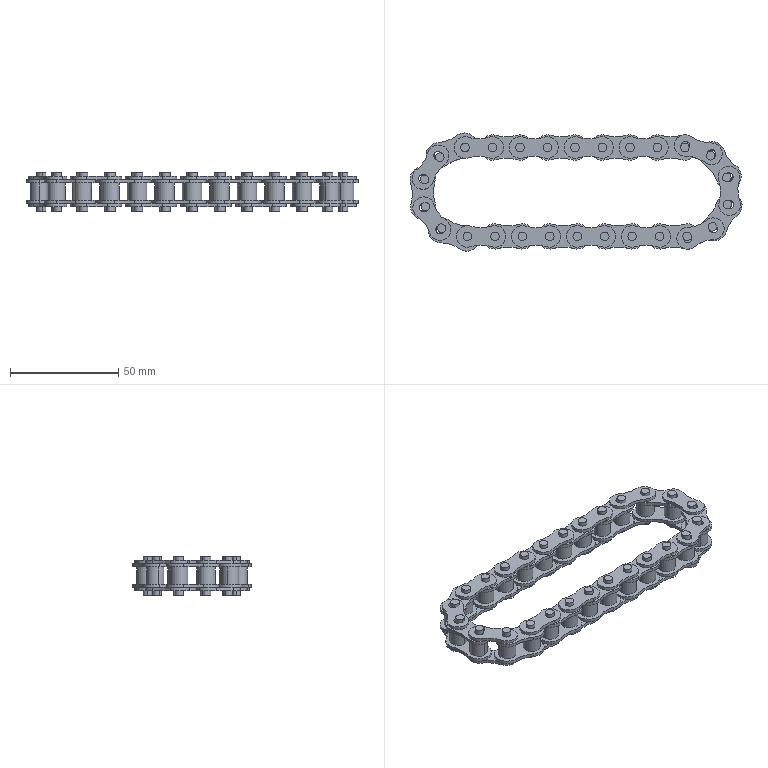Part | NX | features BREP 105 | 105 solids | 836 faces | box 153.555 x 54.676 x 17.95 mm | volume 28533 mm3 | cylinder 626 | plane 210 | commonest cylinder face diameters 3.97 x314 30 x104 10 x78 11.7 x78 7.92 x52